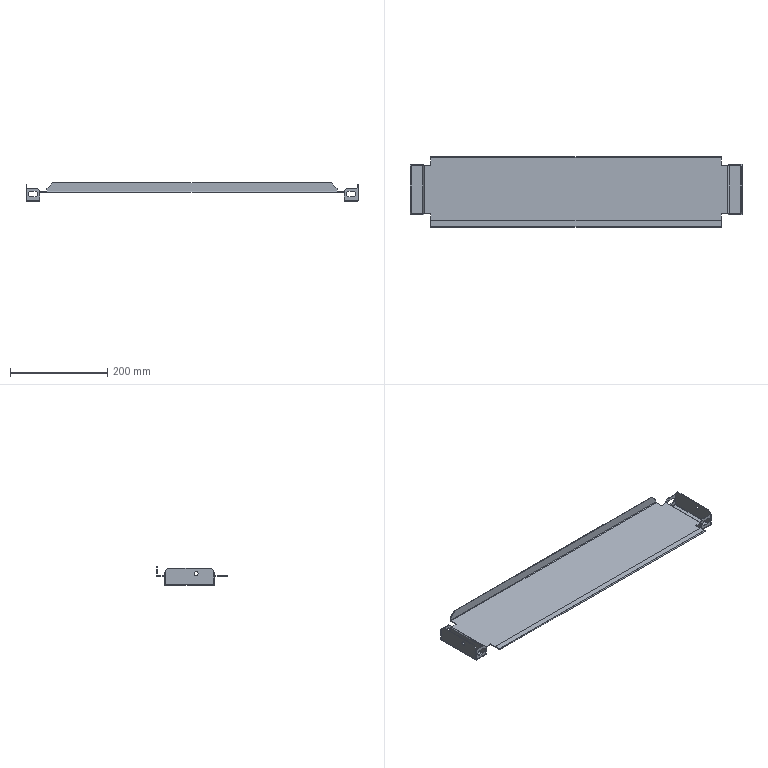Part | STEP file | 8XS320011-1~2_8XS320011.2 | 1 solid | 140 faces | box 682 x 145 x 38.3 mm | volume 150091 mm3 | plane 88 | cylinder 36 | spline 16 | commonest cylinder face diameters 2 x11 4.4 x11 12 x8 8 x4 0.1 x1 2.5 x1